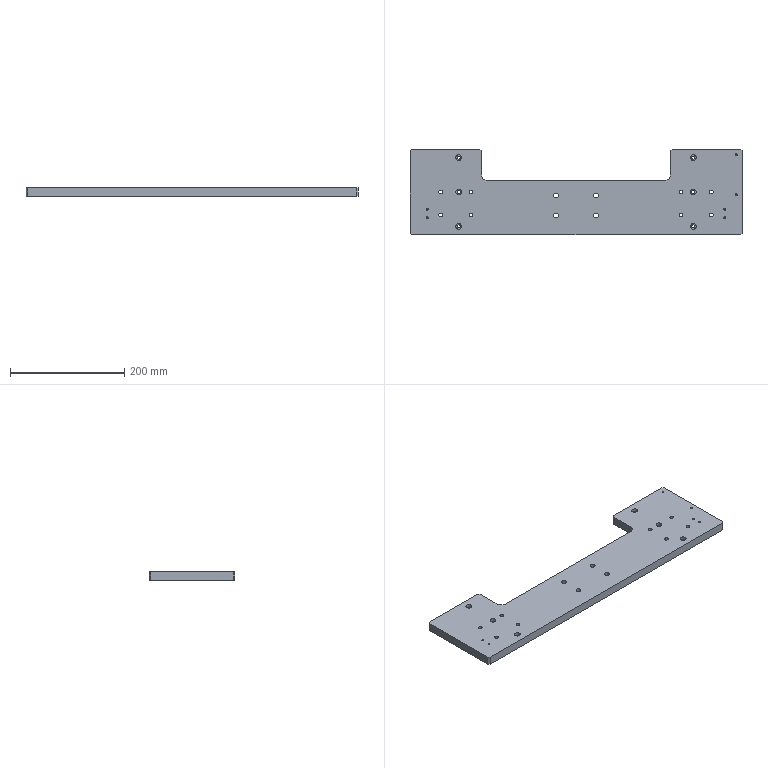Part | NX | 1 solid | 100 faces | box 580 x 150 x 15 mm | volume 1013315 mm3 | cylinder 52 | plane 34 | cone 14 | commonest cylinder face diameters 3.3 x10 6.6 x8 11 x8 5.5 x6 10 x6 4.2 x4